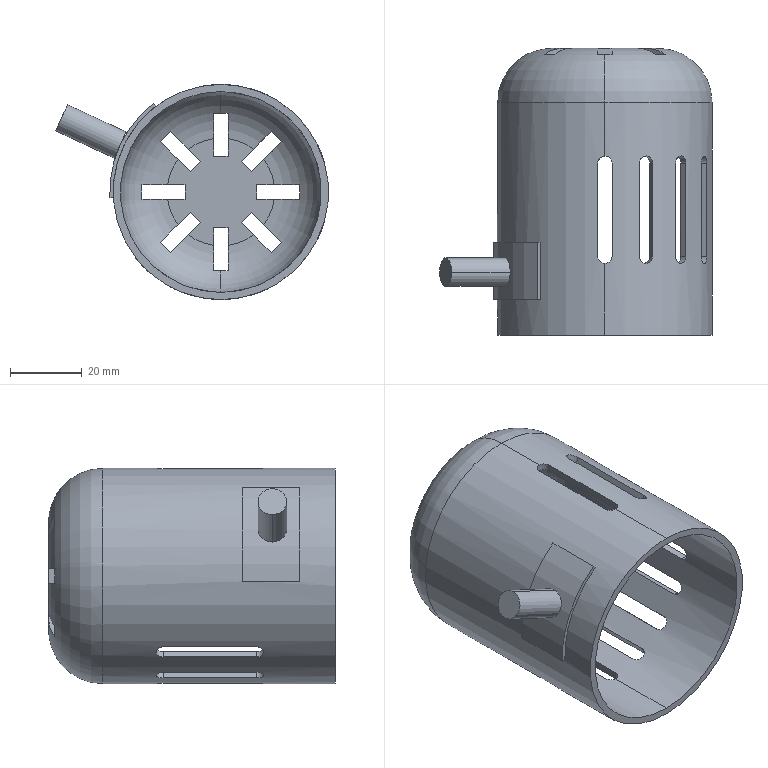Part | SolidWorks | features ICE 4, CirPattern 1, Extrusion 1, Fillet 1, Shell 1 | 2 solids | 96 faces | box 76.1 x 80 x 60 mm | volume 29738 mm3 | plane 63 | cylinder 29 | torus 4 | commonest cylinder face diameters 4 x22 8 x2 56 x2 60 x2 62 x1